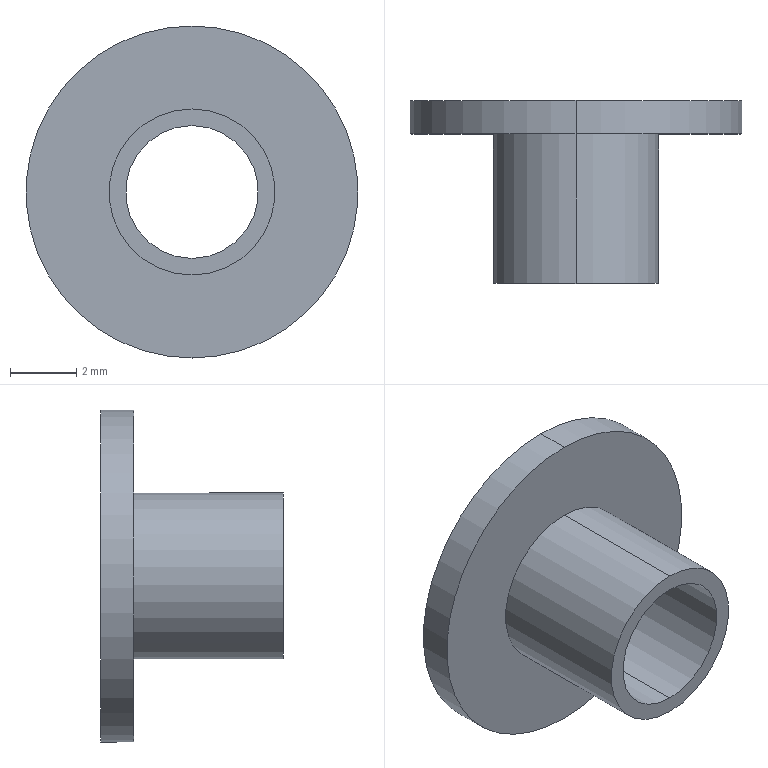Part | SolidWorks | features Revolution 1 | 1 solid | 9 faces | box 10 x 5.5 x 10 mm | volume 97.782 mm3 | cylinder 6 | plane 3 | commonest cylinder face diameters 4 x2 5 x2 10 x2
STEP:
#1=CARTESIAN_POINT('',(0.,4.5,-2.5));
#2=VERTEX_POINT('',#1);
#3=CARTESIAN_POINT('',(0.,4.5,2.5));
#4=VERTEX_POINT('',#3);
#5=CARTESIAN_POINT('',(0.,4.5,0.));
#6=DIRECTION('',(0.,-1.,0.));
#7=DIRECTION('',(0.,0.,-1.));
#8=AXIS2_PLACEMENT_3D('',#5,#6,#7);
#9=CIRCLE('',#8,2.5);
#10=EDGE_CURVE('',#2,#4,#9,.T.);
#11=ORIENTED_EDGE('',*,*,#10,.T.);
#12=CARTESIAN_POINT('',(0.,0.,2.5));
#13=VERTEX_POINT('',#12);
#14=CARTESIAN_POINT('',(0.,0.,2.5));
#15=DIRECTION('',(0.,-1.,0.));
#16=VECTOR('',#15,1000.);
#17=LINE('',#14,#16);
#18=EDGE_CURVE('',#4,#13,#17,.T.);
#19=ORIENTED_EDGE('',*,*,#18,.T.);
#20=CARTESIAN_POINT('',(0.,0.,-2.5));
#21=VERTEX_POINT('',#20);
#22=CARTESIAN_POINT('',(0.,0.,0.));
#23=DIRECTION('',(0.,-1.,0.));
#24=DIRECTION('',(0.,0.,-1.));
#25=AXIS2_PLACEMENT_3D('',#22,#23,#24);
#26=CIRCLE('',#25,2.5);
#27=EDGE_CURVE('',#21,#13,#26,.T.);
#28=ORIENTED_EDGE('',*,*,#27,.F.);
#29=CARTESIAN_POINT('',(0.,0.,-2.5));
#30=DIRECTION('',(0.,-1.,0.));
#31=VECTOR('',#30,1000.);
#32=LINE('',#29,#31);
#33=EDGE_CURVE('',#2,#21,#32,.T.);
#34=ORIENTED_EDGE('',*,*,#33,.F.);
#35=EDGE_LOOP('',(#11,#19,#28,#34));
#36=FACE_OUTER_BOUND('',#35,.T.);
#37=CARTESIAN_POINT('',(0.,0.,0.));
#38=DIRECTION('',(0.,-1.,0.));
#39=DIRECTION('',(0.,0.,-1.));
#40=AXIS2_PLACEMENT_3D('',#37,#38,#39);
#41=CYLINDRICAL_SURFACE('',#40,2.5);
#42=ADVANCED_FACE('',(#36),#41,.T.);
#43=CARTESIAN_POINT('',(0.,5.5,-5.));
#44=VERTEX_POINT('',#43);
#45=CARTESIAN_POINT('',(0.,5.5,5.));
#46=VERTEX_POINT('',#45);
#47=CARTESIAN_POINT('',(0.,5.5,0.));
#48=DIRECTION('',(0.,-1.,0.));
#49=DIRECTION('',(0.,0.,-1.));
#50=AXIS2_PLACEMENT_3D('',#47,#48,#49);
#51=CIRCLE('',#50,5.);
#52=EDGE_CURVE('',#44,#46,#51,.T.);
#53=ORIENTED_EDGE('',*,*,#52,.T.);
#54=CARTESIAN_POINT('',(0.,4.5,5.));
#55=VERTEX_POINT('',#54);
#56=CARTESIAN_POINT('',(0.,0.,5.));
#57=DIRECTION('',(0.,-1.,0.));
#58=VECTOR('',#57,1000.);
#59=LINE('',#56,#58);
#60=EDGE_CURVE('',#46,#55,#59,.T.);
#61=ORIENTED_EDGE('',*,*,#60,.T.);
#62=CARTESIAN_POINT('',(0.,4.5,-5.));
#63=VERTEX_POINT('',#62);
#64=CARTESIAN_POINT('',(0.,4.5,0.));
#65=DIRECTION('',(0.,-1.,0.));
#66=DIRECTION('',(0.,0.,-1.));
#67=AXIS2_PLACEMENT_3D('',#64,#65,#66);
#68=CIRCLE('',#67,5.);
#69=EDGE_CURVE('',#63,#55,#68,.T.);
#70=ORIENTED_EDGE('',*,*,#69,.F.);
#71=CARTESIAN_POINT('',(0.,0.,-5.));
#72=DIRECTION('',(0.,-1.,0.));
#73=VECTOR('',#72,1000.);
#74=LINE('',#71,#73);
#75=EDGE_CURVE('',#44,#63,#74,.T.);
#76=ORIENTED_EDGE('',*,*,#75,.F.);
#77=EDGE_LOOP('',(#53,#61,#70,#76));
#78=FACE_OUTER_BOUND('',#77,.T.);
#79=CARTESIAN_POINT('',(0.,0.,0.));
#80=DIRECTION('',(0.,-1.,0.));
#81=DIRECTION('',(0.,0.,-1.));
#82=AXIS2_PLACEMENT_3D('',#79,#80,#81);
#83=CYLINDRICAL_SURFACE('',#82,5.);
#84=ADVANCED_FACE('',(#78),#83,.T.);
#85=CARTESIAN_POINT('',(0.,5.5,2.));
#86=VERTEX_POINT('',#85);
#87=CARTESIAN_POINT('',(0.,5.5,-2.));
#88=VERTEX_POINT('',#87);
#89=CARTESIAN_POINT('',(0.,5.5,0.));
#90=DIRECTION('',(0.,-1.,0.));
#91=DIRECTION('',(0.,0.,-1.));
#92=AXIS2_PLACEMENT_3D('',#89,#90,#91);
#93=CIRCLE('',#92,2.);
#94=EDGE_CURVE('',#86,#88,#93,.T.);
#95=ORIENTED_EDGE('',*,*,#94,.F.);
#96=CARTESIAN_POINT('',(0.,0.,2.));
#97=VERTEX_POINT('',#96);
#98=CARTESIAN_POINT('',(0.,0.,2.));
#99=DIRECTION('',(0.,-1.,0.));
#100=VECTOR('',#99,1000.);
#101=LINE('',#98,#100);
#102=EDGE_CURVE('',#86,#97,#101,.T.);
#103=ORIENTED_EDGE('',*,*,#102,.T.);
#104=CARTESIAN_POINT('',(0.,0.,-2.));
#105=VERTEX_POINT('',#104);
#106=CARTESIAN_POINT('',(0.,0.,0.));
#107=DIRECTION('',(0.,-1.,0.));
#108=DIRECTION('',(0.,0.,-1.));
#109=AXIS2_PLACEMENT_3D('',#106,#107,#108);
#110=CIRCLE('',#109,2.);
#111=EDGE_CURVE('',#97,#105,#110,.T.);
#112=ORIENTED_EDGE('',*,*,#111,.T.);
#113=CARTESIAN_POINT('',(0.,0.,-2.));
#114=DIRECTION('',(0.,-1.,0.));
#115=VECTOR('',#114,1000.);
#116=LINE('',#113,#115);
#117=EDGE_CURVE('',#88,#105,#116,.T.);
#118=ORIENTED_EDGE('',*,*,#117,.F.);
#119=EDGE_LOOP('',(#95,#103,#112,#118));
#120=FACE_OUTER_BOUND('',#119,.T.);
#121=CARTESIAN_POINT('',(0.,0.,0.));
#122=DIRECTION('',(0.,-1.,0.));
#123=DIRECTION('',(0.,0.,-1.));
#124=AXIS2_PLACEMENT_3D('',#121,#122,#123);
#125=CYLINDRICAL_SURFACE('',#124,2.);
#126=ADVANCED_FACE('',(#120),#125,.F.);
#127=ORIENTED_EDGE('',*,*,#102,.F.);
#128=CARTESIAN_POINT('',(0.,5.5,0.));
#129=DIRECTION('',(0.,-1.,0.));
#130=DIRECTION('',(0.,0.,-1.));
#131=AXIS2_PLACEMENT_3D('',#128,#129,#130);
#132=CIRCLE('',#131,2.);
#133=EDGE_CURVE('',#88,#86,#132,.T.);
#134=ORIENTED_EDGE('',*,*,#133,.F.);
#135=ORIENTED_EDGE('',*,*,#117,.T.);
#136=CARTESIAN_POINT('',(0.,0.,0.));
#137=DIRECTION('',(0.,-1.,0.));
#138=DIRECTION('',(0.,0.,-1.));
#139=AXIS2_PLACEMENT_3D('',#136,#137,#138);
#140=CIRCLE('',#139,2.);
#141=EDGE_CURVE('',#105,#97,#140,.T.);
#142=ORIENTED_EDGE('',*,*,#141,.T.);
#143=EDGE_LOOP('',(#127,#134,#135,#142));
#144=FACE_OUTER_BOUND('',#143,.T.);
#145=CARTESIAN_POINT('',(0.,0.,0.));
#146=DIRECTION('',(0.,-1.,0.));
#147=DIRECTION('',(0.,0.,-1.));
#148=AXIS2_PLACEMENT_3D('',#145,#146,#147);
#149=CYLINDRICAL_SURFACE('',#148,2.);
#150=ADVANCED_FACE('',(#144),#149,.F.);
#151=ORIENTED_EDGE('',*,*,#133,.T.);
#152=ORIENTED_EDGE('',*,*,#94,.T.);
#153=EDGE_LOOP('',(#151,#152));
#154=FACE_BOUND('',#153,.T.);
#155=ORIENTED_EDGE('',*,*,#52,.F.);
#156=CARTESIAN_POINT('',(0.,5.5,0.));
#157=DIRECTION('',(0.,-1.,0.));
#158=DIRECTION('',(0.,0.,-1.));
#159=AXIS2_PLACEMENT_3D('',#156,#157,#158);
#160=CIRCLE('',#159,5.);
#161=EDGE_CURVE('',#46,#44,#160,.T.);
#162=ORIENTED_EDGE('',*,*,#161,.F.);
#163=EDGE_LOOP('',(#155,#162));
#164=FACE_OUTER_BOUND('',#163,.T.);
#165=CARTESIAN_POINT('',(2.,5.5,0.));
#166=DIRECTION('',(0.,1.,0.));
#167=DIRECTION('',(0.,0.,1.));
#168=AXIS2_PLACEMENT_3D('',#165,#166,#167);
#169=PLANE('',#168);
#170=ADVANCED_FACE('',(#154,#164),#169,.T.);
#171=ORIENTED_EDGE('',*,*,#60,.F.);
#172=ORIENTED_EDGE('',*,*,#161,.T.);
#173=ORIENTED_EDGE('',*,*,#75,.T.);
#174=CARTESIAN_POINT('',(0.,4.5,0.));
#175=DIRECTION('',(0.,-1.,0.));
#176=DIRECTION('',(0.,0.,-1.));
#177=AXIS2_PLACEMENT_3D('',#174,#175,#176);
#178=CIRCLE('',#177,5.);
#179=EDGE_CURVE('',#55,#63,#178,.T.);
#180=ORIENTED_EDGE('',*,*,#179,.F.);
#181=EDGE_LOOP('',(#171,#172,#173,#180));
#182=FACE_OUTER_BOUND('',#181,.T.);
#183=CARTESIAN_POINT('',(0.,0.,0.));
#184=DIRECTION('',(0.,-1.,0.));
#185=DIRECTION('',(0.,0.,-1.));
#186=AXIS2_PLACEMENT_3D('',#183,#184,#185);
#187=CYLINDRICAL_SURFACE('',#186,5.);
#188=ADVANCED_FACE('',(#182),#187,.T.);
#189=ORIENTED_EDGE('',*,*,#69,.T.);
#190=ORIENTED_EDGE('',*,*,#179,.T.);
#191=EDGE_LOOP('',(#189,#190));
#192=FACE_OUTER_BOUND('',#191,.T.);
#193=ORIENTED_EDGE('',*,*,#10,.F.);
#194=CARTESIAN_POINT('',(0.,4.5,0.));
#195=DIRECTION('',(0.,-1.,0.));
#196=DIRECTION('',(0.,0.,-1.));
#197=AXIS2_PLACEMENT_3D('',#194,#195,#196);
#198=CIRCLE('',#197,2.5);
#199=EDGE_CURVE('',#4,#2,#198,.T.);
#200=ORIENTED_EDGE('',*,*,#199,.F.);
#201=EDGE_LOOP('',(#193,#200));
#202=FACE_BOUND('',#201,.T.);
#203=CARTESIAN_POINT('',(5.,4.5,0.));
#204=DIRECTION('',(0.,-1.,0.));
#205=DIRECTION('',(0.,0.,-1.));
#206=AXIS2_PLACEMENT_3D('',#203,#204,#205);
#207=PLANE('',#206);
#208=ADVANCED_FACE('',(#192,#202),#207,.T.);
#209=ORIENTED_EDGE('',*,*,#18,.F.);
#210=ORIENTED_EDGE('',*,*,#199,.T.);
#211=ORIENTED_EDGE('',*,*,#33,.T.);
#212=CARTESIAN_POINT('',(0.,0.,0.));
#213=DIRECTION('',(0.,-1.,0.));
#214=DIRECTION('',(0.,0.,-1.));
#215=AXIS2_PLACEMENT_3D('',#212,#213,#214);
#216=CIRCLE('',#215,2.5);
#217=EDGE_CURVE('',#13,#21,#216,.T.);
#218=ORIENTED_EDGE('',*,*,#217,.F.);
#219=EDGE_LOOP('',(#209,#210,#211,#218));
#220=FACE_OUTER_BOUND('',#219,.T.);
#221=CARTESIAN_POINT('',(0.,0.,0.));
#222=DIRECTION('',(0.,-1.,0.));
#223=DIRECTION('',(0.,0.,-1.));
#224=AXIS2_PLACEMENT_3D('',#221,#222,#223);
#225=CYLINDRICAL_SURFACE('',#224,2.5);
#226=ADVANCED_FACE('',(#220),#225,.T.);
#227=ORIENTED_EDGE('',*,*,#27,.T.);
#228=ORIENTED_EDGE('',*,*,#217,.T.);
#229=EDGE_LOOP('',(#227,#228));
#230=FACE_OUTER_BOUND('',#229,.T.);
#231=ORIENTED_EDGE('',*,*,#141,.F.);
#232=ORIENTED_EDGE('',*,*,#111,.F.);
#233=EDGE_LOOP('',(#231,#232));
#234=FACE_BOUND('',#233,.T.);
#235=CARTESIAN_POINT('',(2.5,0.,0.));
#236=DIRECTION('',(0.,-1.,0.));
#237=DIRECTION('',(0.,0.,-1.));
#238=AXIS2_PLACEMENT_3D('',#235,#236,#237);
#239=PLANE('',#238);
#240=ADVANCED_FACE('',(#230,#234),#239,.T.);
#241=CLOSED_SHELL('',(#42,#84,#126,#150,#170,#188,#208,#226,#240));
#242=MANIFOLD_SOLID_BREP('',#241);
#243=CARTESIAN_POINT('',(0.,0.,0.));
#244=DIRECTION('',(0.,0.,1.));
#245=DIRECTION('',(1.,0.,0.));
#246=AXIS2_PLACEMENT_3D('',#243,#244,#245);
#247=(LENGTH_UNIT()NAMED_UNIT(*)SI_UNIT(.MILLI.,.METRE.));
#248=UNCERTAINTY_MEASURE_WITH_UNIT(LENGTH_MEASURE(0.00001),#247,'','');
#249=(NAMED_UNIT(*)PLANE_ANGLE_UNIT()SI_UNIT($,.RADIAN.));
#250=(NAMED_UNIT(*)SI_UNIT($,.STERADIAN.)SOLID_ANGLE_UNIT());
#251=(GEOMETRIC_REPRESENTATION_CONTEXT(3)GLOBAL_UNCERTAINTY_ASSIGNED_CONTEXT((#248))GLOBAL_UNIT_ASSIGNED_CONTEXT((#247,#249,#250))REPRESENTATION_CONTEXT('',''));
#252=ADVANCED_BREP_SHAPE_REPRESENTATION('',(#242,#246),#251);